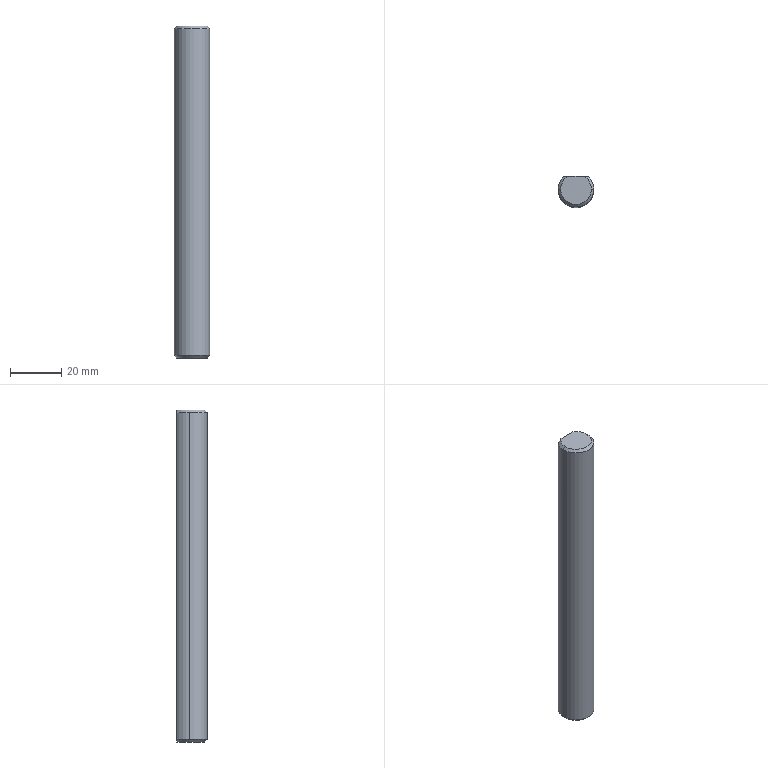Part | STEP file | BPSP-03-014 Sliding Rib_Default | 1 solid | 24 faces | box 14 x 12 x 130 mm | volume 17958 mm3 | cone 12 | cylinder 9 | plane 3 | commonest cylinder face diameters 3.3 x6 14 x3